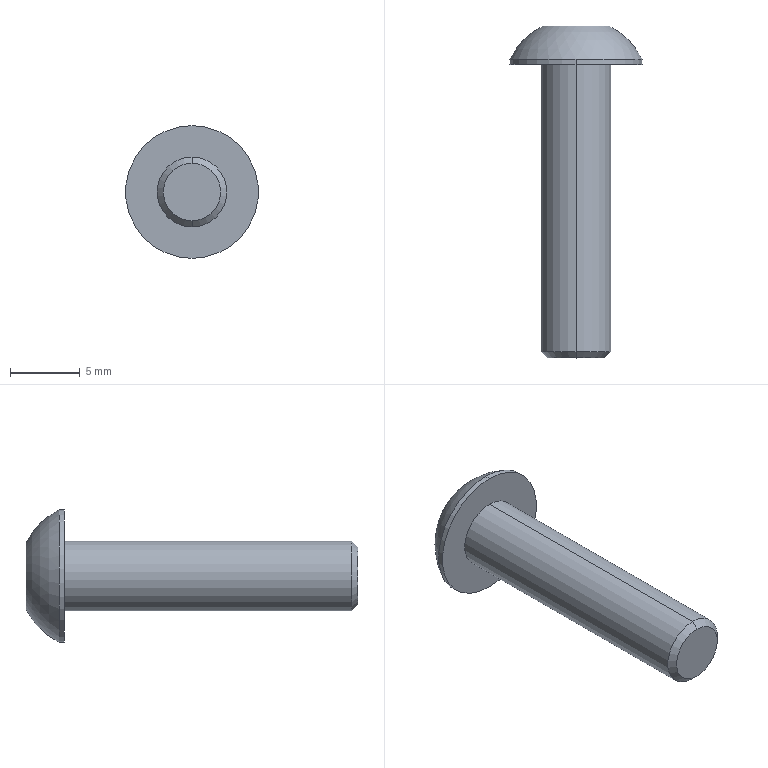Part | SolidWorks | features BaseBody 1 | 1 solid | 17 faces | box 9.5 x 23.75 x 9.5 mm | volume 537.038 mm3 | plane 10 | cylinder 4 | cone 2 | sphere 1 | commonest cylinder face diameters 5 x2 9.5 x2
STEP:
#1=CARTESIAN_POINT('',(0.,-21.,-2.055));
#2=VERTEX_POINT('',#1);
#3=CARTESIAN_POINT('',(0.,-21.,2.055));
#4=VERTEX_POINT('',#3);
#5=CARTESIAN_POINT('',(0.,-21.,0.));
#6=DIRECTION('',(0.,-1.,0.));
#7=DIRECTION('',(0.,0.,-1.));
#8=AXIS2_PLACEMENT_3D('',#5,#6,#7);
#9=CIRCLE('',#8,2.055);
#10=EDGE_CURVE('',#2,#4,#9,.T.);
#11=ORIENTED_EDGE('',*,*,#10,.F.);
#12=CARTESIAN_POINT('',(0.,-20.555,-2.5));
#13=VERTEX_POINT('',#12);
#14=CARTESIAN_POINT('',(0.,-21.,-2.055));
#15=DIRECTION('',(0.,0.7071,-0.7071));
#16=VECTOR('',#15,1000.);
#17=LINE('',#14,#16);
#18=EDGE_CURVE('',#2,#13,#17,.T.);
#19=ORIENTED_EDGE('',*,*,#18,.T.);
#20=CARTESIAN_POINT('',(0.,-20.555,2.5));
#21=VERTEX_POINT('',#20);
#22=CARTESIAN_POINT('',(0.,-20.555,0.));
#23=DIRECTION('',(0.,1.,0.));
#24=DIRECTION('',(0.,0.,-1.));
#25=AXIS2_PLACEMENT_3D('',#22,#23,#24);
#26=CIRCLE('',#25,2.5);
#27=EDGE_CURVE('',#21,#13,#26,.T.);
#28=ORIENTED_EDGE('',*,*,#27,.F.);
#29=CARTESIAN_POINT('',(0.,-21.,2.055));
#30=DIRECTION('',(0.,0.7071,0.7071));
#31=VECTOR('',#30,1000.);
#32=LINE('',#29,#31);
#33=EDGE_CURVE('',#4,#21,#32,.T.);
#34=ORIENTED_EDGE('',*,*,#33,.F.);
#35=EDGE_LOOP('',(#11,#19,#28,#34));
#36=FACE_OUTER_BOUND('',#35,.T.);
#37=CARTESIAN_POINT('',(0.,-21.,0.));
#38=DIRECTION('',(0.,1.,0.));
#39=DIRECTION('',(0.,0.,1.));
#40=AXIS2_PLACEMENT_3D('',#37,#38,#39);
#41=CONICAL_SURFACE('',#40,2.055,0.7854);
#42=ADVANCED_FACE('',(#36),#41,.T.);
#43=ORIENTED_EDGE('',*,*,#27,.T.);
#44=CARTESIAN_POINT('',(0.,0.,-2.5));
#45=VERTEX_POINT('',#44);
#46=CARTESIAN_POINT('',(0.,-21.,-2.5));
#47=DIRECTION('',(0.,1.,0.));
#48=VECTOR('',#47,1000.);
#49=LINE('',#46,#48);
#50=EDGE_CURVE('',#13,#45,#49,.T.);
#51=ORIENTED_EDGE('',*,*,#50,.T.);
#52=CARTESIAN_POINT('',(0.,0.,2.5));
#53=VERTEX_POINT('',#52);
#54=CARTESIAN_POINT('',(0.,0.,0.));
#55=DIRECTION('',(0.,-1.,0.));
#56=DIRECTION('',(0.,0.,1.));
#57=AXIS2_PLACEMENT_3D('',#54,#55,#56);
#58=CIRCLE('',#57,2.5);
#59=EDGE_CURVE('',#45,#53,#58,.T.);
#60=ORIENTED_EDGE('',*,*,#59,.T.);
#61=CARTESIAN_POINT('',(0.,-21.,2.5));
#62=DIRECTION('',(0.,1.,0.));
#63=VECTOR('',#62,1000.);
#64=LINE('',#61,#63);
#65=EDGE_CURVE('',#21,#53,#64,.T.);
#66=ORIENTED_EDGE('',*,*,#65,.F.);
#67=EDGE_LOOP('',(#43,#51,#60,#66));
#68=FACE_OUTER_BOUND('',#67,.T.);
#69=CARTESIAN_POINT('',(0.,-21.,0.));
#70=DIRECTION('',(0.,1.,0.));
#71=DIRECTION('',(0.,0.,1.));
#72=AXIS2_PLACEMENT_3D('',#69,#70,#71);
#73=CYLINDRICAL_SURFACE('',#72,2.5);
#74=ADVANCED_FACE('',(#68),#73,.T.);
#75=CARTESIAN_POINT('',(0.,0.38,-4.75));
#76=VERTEX_POINT('',#75);
#77=CARTESIAN_POINT('',(0.,0.38,4.75));
#78=VERTEX_POINT('',#77);
#79=CARTESIAN_POINT('',(0.,0.38,0.));
#80=DIRECTION('',(0.,-1.,0.));
#81=DIRECTION('',(0.,0.,-1.));
#82=AXIS2_PLACEMENT_3D('',#79,#80,#81);
#83=CIRCLE('',#82,4.75);
#84=EDGE_CURVE('',#76,#78,#83,.T.);
#85=ORIENTED_EDGE('',*,*,#84,.T.);
#86=CARTESIAN_POINT('',(0.,0.,4.75));
#87=VERTEX_POINT('',#86);
#88=CARTESIAN_POINT('',(0.,2.75,4.75));
#89=DIRECTION('',(0.,-1.,0.));
#90=VECTOR('',#89,1000.);
#91=LINE('',#88,#90);
#92=EDGE_CURVE('',#78,#87,#91,.T.);
#93=ORIENTED_EDGE('',*,*,#92,.T.);
#94=CARTESIAN_POINT('',(0.,0.,-4.75));
#95=VERTEX_POINT('',#94);
#96=CARTESIAN_POINT('',(0.,0.,0.));
#97=DIRECTION('',(0.,1.,0.));
#98=DIRECTION('',(0.,0.,1.));
#99=AXIS2_PLACEMENT_3D('',#96,#97,#98);
#100=CIRCLE('',#99,4.75);
#101=EDGE_CURVE('',#87,#95,#100,.T.);
#102=ORIENTED_EDGE('',*,*,#101,.T.);
#103=CARTESIAN_POINT('',(0.,2.75,-4.75));
#104=DIRECTION('',(0.,-1.,0.));
#105=VECTOR('',#104,1000.);
#106=LINE('',#103,#105);
#107=EDGE_CURVE('',#76,#95,#106,.T.);
#108=ORIENTED_EDGE('',*,*,#107,.F.);
#109=EDGE_LOOP('',(#85,#93,#102,#108));
#110=FACE_OUTER_BOUND('',#109,.T.);
#111=CARTESIAN_POINT('',(0.,2.75,0.));
#112=DIRECTION('',(0.,-1.,0.));
#113=DIRECTION('',(0.,0.,-1.));
#114=AXIS2_PLACEMENT_3D('',#111,#112,#113);
#115=CYLINDRICAL_SURFACE('',#114,4.75);
#116=ADVANCED_FACE('',(#110),#115,.T.);
#117=CARTESIAN_POINT('',(0.8862,2.75,1.535));
#118=VERTEX_POINT('',#117);
#119=CARTESIAN_POINT('',(1.772,2.75,0.));
#120=VERTEX_POINT('',#119);
#121=CARTESIAN_POINT('',(0.8862,2.75,1.535));
#122=DIRECTION('',(0.5,0.,-0.866));
#123=VECTOR('',#122,1000.);
#124=LINE('',#121,#123);
#125=EDGE_CURVE('',#118,#120,#124,.T.);
#126=ORIENTED_EDGE('',*,*,#125,.F.);
#127=CARTESIAN_POINT('',(-0.8862,2.75,1.535));
#128=VERTEX_POINT('',#127);
#129=CARTESIAN_POINT('',(-0.8862,2.75,1.535));
#130=DIRECTION('',(1.,0.,0.));
#131=VECTOR('',#130,1000.);
#132=LINE('',#129,#131);
#133=EDGE_CURVE('',#128,#118,#132,.T.);
#134=ORIENTED_EDGE('',*,*,#133,.F.);
#135=CARTESIAN_POINT('',(-1.772,2.75,0.));
#136=VERTEX_POINT('',#135);
#137=CARTESIAN_POINT('',(-1.772,2.75,0.));
#138=DIRECTION('',(0.5,0.,0.866));
#139=VECTOR('',#138,1000.);
#140=LINE('',#137,#139);
#141=EDGE_CURVE('',#136,#128,#140,.T.);
#142=ORIENTED_EDGE('',*,*,#141,.F.);
#143=CARTESIAN_POINT('',(-0.8862,2.75,-1.535));
#144=VERTEX_POINT('',#143);
#145=CARTESIAN_POINT('',(-0.8862,2.75,-1.535));
#146=DIRECTION('',(-0.5,0.,0.866));
#147=VECTOR('',#146,1000.);
#148=LINE('',#145,#147);
#149=EDGE_CURVE('',#144,#136,#148,.T.);
#150=ORIENTED_EDGE('',*,*,#149,.F.);
#151=CARTESIAN_POINT('',(0.8862,2.75,-1.535));
#152=VERTEX_POINT('',#151);
#153=CARTESIAN_POINT('',(0.8862,2.75,-1.535));
#154=DIRECTION('',(-1.,0.,0.));
#155=VECTOR('',#154,1000.);
#156=LINE('',#153,#155);
#157=EDGE_CURVE('',#152,#144,#156,.T.);
#158=ORIENTED_EDGE('',*,*,#157,.F.);
#159=CARTESIAN_POINT('',(1.772,2.75,0.));
#160=DIRECTION('',(-0.5,0.,-0.866));
#161=VECTOR('',#160,1000.);
#162=LINE('',#159,#161);
#163=EDGE_CURVE('',#120,#152,#162,.T.);
#164=ORIENTED_EDGE('',*,*,#163,.F.);
#165=EDGE_LOOP('',(#126,#134,#142,#150,#158,#164));
#166=FACE_BOUND('',#165,.T.);
#167=CARTESIAN_POINT('',(0.,2.75,-2.375));
#168=VERTEX_POINT('',#167);
#169=CARTESIAN_POINT('',(0.,2.75,2.375));
#170=VERTEX_POINT('',#169);
#171=CARTESIAN_POINT('',(0.,2.75,0.));
#172=DIRECTION('',(0.,-1.,0.));
#173=DIRECTION('',(0.,0.,-1.));
#174=AXIS2_PLACEMENT_3D('',#171,#172,#173);
#175=CIRCLE('',#174,2.375);
#176=EDGE_CURVE('',#168,#170,#175,.T.);
#177=ORIENTED_EDGE('',*,*,#176,.F.);
#178=CARTESIAN_POINT('',(0.,2.75,0.));
#179=DIRECTION('',(0.,-1.,0.));
#180=DIRECTION('',(0.,0.,-1.));
#181=AXIS2_PLACEMENT_3D('',#178,#179,#180);
#182=CIRCLE('',#181,2.375);
#183=EDGE_CURVE('',#170,#168,#182,.T.);
#184=ORIENTED_EDGE('',*,*,#183,.F.);
#185=EDGE_LOOP('',(#177,#184));
#186=FACE_OUTER_BOUND('',#185,.T.);
#187=CARTESIAN_POINT('',(0.,2.75,0.));
#188=DIRECTION('',(0.,1.,0.));
#189=DIRECTION('',(1.,0.,0.));
#190=AXIS2_PLACEMENT_3D('',#187,#188,#189);
#191=PLANE('',#190);
#192=ADVANCED_FACE('',(#166,#186),#191,.T.);
#193=ORIENTED_EDGE('',*,*,#125,.T.);
#194=CARTESIAN_POINT('',(1.772,1.19,0.));
#195=VERTEX_POINT('',#194);
#196=CARTESIAN_POINT('',(1.772,1.19,0.));
#197=DIRECTION('',(0.,1.,0.));
#198=VECTOR('',#197,1000.);
#199=LINE('',#196,#198);
#200=EDGE_CURVE('',#195,#120,#199,.T.);
#201=ORIENTED_EDGE('',*,*,#200,.F.);
#202=CARTESIAN_POINT('',(0.8862,1.19,1.535));
#203=VERTEX_POINT('',#202);
#204=CARTESIAN_POINT('',(0.8862,1.19,1.535));
#205=DIRECTION('',(0.5,0.,-0.866));
#206=VECTOR('',#205,1000.);
#207=LINE('',#204,#206);
#208=EDGE_CURVE('',#203,#195,#207,.T.);
#209=ORIENTED_EDGE('',*,*,#208,.F.);
#210=CARTESIAN_POINT('',(0.8862,1.19,1.535));
#211=DIRECTION('',(0.,1.,0.));
#212=VECTOR('',#211,1000.);
#213=LINE('',#210,#212);
#214=EDGE_CURVE('',#203,#118,#213,.T.);
#215=ORIENTED_EDGE('',*,*,#214,.T.);
#216=EDGE_LOOP('',(#193,#201,#209,#215));
#217=FACE_OUTER_BOUND('',#216,.T.);
#218=CARTESIAN_POINT('',(0.8862,1.19,1.535));
#219=DIRECTION('',(0.866,0.,0.5));
#220=DIRECTION('',(0.,-1.,0.));
#221=AXIS2_PLACEMENT_3D('',#218,#219,#220);
#222=PLANE('',#221);
#223=ADVANCED_FACE('',(#217),#222,.F.);
#224=ORIENTED_EDGE('',*,*,#133,.T.);
#225=ORIENTED_EDGE('',*,*,#214,.F.);
#226=CARTESIAN_POINT('',(-0.8862,1.19,1.535));
#227=VERTEX_POINT('',#226);
#228=CARTESIAN_POINT('',(-0.8862,1.19,1.535));
#229=DIRECTION('',(1.,0.,0.));
#230=VECTOR('',#229,1000.);
#231=LINE('',#228,#230);
#232=EDGE_CURVE('',#227,#203,#231,.T.);
#233=ORIENTED_EDGE('',*,*,#232,.F.);
#234=CARTESIAN_POINT('',(-0.8862,1.19,1.535));
#235=DIRECTION('',(0.,1.,0.));
#236=VECTOR('',#235,1000.);
#237=LINE('',#234,#236);
#238=EDGE_CURVE('',#227,#128,#237,.T.);
#239=ORIENTED_EDGE('',*,*,#238,.T.);
#240=EDGE_LOOP('',(#224,#225,#233,#239));
#241=FACE_OUTER_BOUND('',#240,.T.);
#242=CARTESIAN_POINT('',(-0.8862,1.19,1.535));
#243=DIRECTION('',(0.,0.,1.));
#244=DIRECTION('',(1.,0.,0.));
#245=AXIS2_PLACEMENT_3D('',#242,#243,#244);
#246=PLANE('',#245);
#247=ADVANCED_FACE('',(#241),#246,.F.);
#248=ORIENTED_EDGE('',*,*,#141,.T.);
#249=ORIENTED_EDGE('',*,*,#238,.F.);
#250=CARTESIAN_POINT('',(-1.772,1.19,0.));
#251=VERTEX_POINT('',#250);
#252=CARTESIAN_POINT('',(-1.772,1.19,0.));
#253=DIRECTION('',(0.5,0.,0.866));
#254=VECTOR('',#253,1000.);
#255=LINE('',#252,#254);
#256=EDGE_CURVE('',#251,#227,#255,.T.);
#257=ORIENTED_EDGE('',*,*,#256,.F.);
#258=CARTESIAN_POINT('',(-1.772,1.19,0.));
#259=DIRECTION('',(0.,1.,0.));
#260=VECTOR('',#259,1000.);
#261=LINE('',#258,#260);
#262=EDGE_CURVE('',#251,#136,#261,.T.);
#263=ORIENTED_EDGE('',*,*,#262,.T.);
#264=EDGE_LOOP('',(#248,#249,#257,#263));
#265=FACE_OUTER_BOUND('',#264,.T.);
#266=CARTESIAN_POINT('',(-1.772,1.19,0.));
#267=DIRECTION('',(-0.866,0.,0.5));
#268=DIRECTION('',(0.,1.,0.));
#269=AXIS2_PLACEMENT_3D('',#266,#267,#268);
#270=PLANE('',#269);
#271=ADVANCED_FACE('',(#265),#270,.F.);
#272=ORIENTED_EDGE('',*,*,#149,.T.);
#273=ORIENTED_EDGE('',*,*,#262,.F.);
#274=CARTESIAN_POINT('',(-0.8862,1.19,-1.535));
#275=VERTEX_POINT('',#274);
#276=CARTESIAN_POINT('',(-0.8862,1.19,-1.535));
#277=DIRECTION('',(-0.5,0.,0.866));
#278=VECTOR('',#277,1000.);
#279=LINE('',#276,#278);
#280=EDGE_CURVE('',#275,#251,#279,.T.);
#281=ORIENTED_EDGE('',*,*,#280,.F.);
#282=CARTESIAN_POINT('',(-0.8862,1.19,-1.535));
#283=DIRECTION('',(0.,1.,0.));
#284=VECTOR('',#283,1000.);
#285=LINE('',#282,#284);
#286=EDGE_CURVE('',#275,#144,#285,.T.);
#287=ORIENTED_EDGE('',*,*,#286,.T.);
#288=EDGE_LOOP('',(#272,#273,#281,#287));
#289=FACE_OUTER_BOUND('',#288,.T.);
#290=CARTESIAN_POINT('',(-0.8862,1.19,-1.535));
#291=DIRECTION('',(-0.866,0.,-0.5));
#292=DIRECTION('',(-0.5,0.,0.866));
#293=AXIS2_PLACEMENT_3D('',#290,#291,#292);
#294=PLANE('',#293);
#295=ADVANCED_FACE('',(#289),#294,.F.);
#296=ORIENTED_EDGE('',*,*,#157,.T.);
#297=ORIENTED_EDGE('',*,*,#286,.F.);
#298=CARTESIAN_POINT('',(0.8862,1.19,-1.535));
#299=VERTEX_POINT('',#298);
#300=CARTESIAN_POINT('',(0.8862,1.19,-1.535));
#301=DIRECTION('',(-1.,0.,0.));
#302=VECTOR('',#301,1000.);
#303=LINE('',#300,#302);
#304=EDGE_CURVE('',#299,#275,#303,.T.);
#305=ORIENTED_EDGE('',*,*,#304,.F.);
#306=CARTESIAN_POINT('',(0.8862,1.19,-1.535));
#307=DIRECTION('',(0.,1.,0.));
#308=VECTOR('',#307,1000.);
#309=LINE('',#306,#308);
#310=EDGE_CURVE('',#299,#152,#309,.T.);
#311=ORIENTED_EDGE('',*,*,#310,.T.);
#312=EDGE_LOOP('',(#296,#297,#305,#311));
#313=FACE_OUTER_BOUND('',#312,.T.);
#314=CARTESIAN_POINT('',(0.8862,1.19,-1.535));
#315=DIRECTION('',(0.,0.,-1.));
#316=DIRECTION('',(-1.,0.,0.));
#317=AXIS2_PLACEMENT_3D('',#314,#315,#316);
#318=PLANE('',#317);
#319=ADVANCED_FACE('',(#313),#318,.F.);
#320=ORIENTED_EDGE('',*,*,#163,.T.);
#321=ORIENTED_EDGE('',*,*,#310,.F.);
#322=CARTESIAN_POINT('',(1.772,1.19,0.));
#323=DIRECTION('',(-0.5,0.,-0.866));
#324=VECTOR('',#323,1000.);
#325=LINE('',#322,#324);
#326=EDGE_CURVE('',#195,#299,#325,.T.);
#327=ORIENTED_EDGE('',*,*,#326,.F.);
#328=ORIENTED_EDGE('',*,*,#200,.T.);
#329=EDGE_LOOP('',(#320,#321,#327,#328));
#330=FACE_OUTER_BOUND('',#329,.T.);
#331=CARTESIAN_POINT('',(1.772,1.19,0.));
#332=DIRECTION('',(0.866,0.,-0.5));
#333=DIRECTION('',(0.,-1.,0.));
#334=AXIS2_PLACEMENT_3D('',#331,#332,#333);
#335=PLANE('',#334);
#336=ADVANCED_FACE('',(#330),#335,.F.);
#337=ORIENTED_EDGE('',*,*,#208,.T.);
#338=ORIENTED_EDGE('',*,*,#326,.T.);
#339=ORIENTED_EDGE('',*,*,#304,.T.);
#340=ORIENTED_EDGE('',*,*,#280,.T.);
#341=ORIENTED_EDGE('',*,*,#256,.T.);
#342=ORIENTED_EDGE('',*,*,#232,.T.);
#343=EDGE_LOOP('',(#337,#338,#339,#340,#341,#342));
#344=FACE_OUTER_BOUND('',#343,.T.);
#345=CARTESIAN_POINT('',(0.,1.19,0.));
#346=DIRECTION('',(0.,1.,0.));
#347=DIRECTION('',(1.,0.,0.));
#348=AXIS2_PLACEMENT_3D('',#345,#346,#347);
#349=PLANE('',#348);
#350=ADVANCED_FACE('',(#344),#349,.T.);
#351=CARTESIAN_POINT('',(0.,-21.,0.));
#352=DIRECTION('',(0.,-1.,0.));
#353=DIRECTION('',(0.,0.,-1.));
#354=AXIS2_PLACEMENT_3D('',#351,#352,#353);
#355=CIRCLE('',#354,2.055);
#356=EDGE_CURVE('',#4,#2,#355,.T.);
#357=ORIENTED_EDGE('',*,*,#356,.T.);
#358=ORIENTED_EDGE('',*,*,#10,.T.);
#359=EDGE_LOOP('',(#357,#358));
#360=FACE_OUTER_BOUND('',#359,.T.);
#361=CARTESIAN_POINT('',(0.,-21.,0.));
#362=DIRECTION('',(0.,-1.,0.));
#363=DIRECTION('',(0.,0.,-1.));
#364=AXIS2_PLACEMENT_3D('',#361,#362,#363);
#365=PLANE('',#364);
#366=ADVANCED_FACE('',(#360),#365,.T.);
#367=CARTESIAN_POINT('',(0.,0.,0.));
#368=DIRECTION('',(0.,-1.,0.));
#369=DIRECTION('',(0.,0.,1.));
#370=AXIS2_PLACEMENT_3D('',#367,#368,#369);
#371=CIRCLE('',#370,2.5);
#372=EDGE_CURVE('',#53,#45,#371,.T.);
#373=ORIENTED_EDGE('',*,*,#372,.F.);
#374=ORIENTED_EDGE('',*,*,#59,.F.);
#375=EDGE_LOOP('',(#373,#374));
#376=FACE_BOUND('',#375,.T.);
#377=CARTESIAN_POINT('',(0.,0.,0.));
#378=DIRECTION('',(0.,1.,0.));
#379=DIRECTION('',(0.,0.,1.));
#380=AXIS2_PLACEMENT_3D('',#377,#378,#379);
#381=CIRCLE('',#380,4.75);
#382=EDGE_CURVE('',#95,#87,#381,.T.);
#383=ORIENTED_EDGE('',*,*,#382,.F.);
#384=ORIENTED_EDGE('',*,*,#101,.F.);
#385=EDGE_LOOP('',(#383,#384));
#386=FACE_OUTER_BOUND('',#385,.T.);
#387=CARTESIAN_POINT('',(0.,0.,0.));
#388=DIRECTION('',(0.,1.,0.));
#389=DIRECTION('',(1.,0.,0.));
#390=AXIS2_PLACEMENT_3D('',#387,#388,#389);
#391=PLANE('',#390);
#392=ADVANCED_FACE('',(#376,#386),#391,.F.);
#393=ORIENTED_EDGE('',*,*,#92,.F.);
#394=CARTESIAN_POINT('',(0.,0.38,0.));
#395=DIRECTION('',(0.,-1.,0.));
#396=DIRECTION('',(0.,0.,-1.));
#397=AXIS2_PLACEMENT_3D('',#394,#395,#396);
#398=CIRCLE('',#397,4.75);
#399=EDGE_CURVE('',#78,#76,#398,.T.);
#400=ORIENTED_EDGE('',*,*,#399,.T.);
#401=ORIENTED_EDGE('',*,*,#107,.T.);
#402=ORIENTED_EDGE('',*,*,#382,.T.);
#403=EDGE_LOOP('',(#393,#400,#401,#402));
#404=FACE_OUTER_BOUND('',#403,.T.);
#405=CARTESIAN_POINT('',(0.,2.75,0.));
#406=DIRECTION('',(0.,-1.,0.));
#407=DIRECTION('',(0.,0.,-1.));
#408=AXIS2_PLACEMENT_3D('',#405,#406,#407);
#409=CYLINDRICAL_SURFACE('',#408,4.75);
#410=ADVANCED_FACE('',(#404),#409,.T.);
#411=ORIENTED_EDGE('',*,*,#50,.F.);
#412=CARTESIAN_POINT('',(0.,-20.555,0.));
#413=DIRECTION('',(0.,1.,0.));
#414=DIRECTION('',(0.,0.,-1.));
#415=AXIS2_PLACEMENT_3D('',#412,#413,#414);
#416=CIRCLE('',#415,2.5);
#417=EDGE_CURVE('',#13,#21,#416,.T.);
#418=ORIENTED_EDGE('',*,*,#417,.T.);
#419=ORIENTED_EDGE('',*,*,#65,.T.);
#420=ORIENTED_EDGE('',*,*,#372,.T.);
#421=EDGE_LOOP('',(#411,#418,#419,#420));
#422=FACE_OUTER_BOUND('',#421,.T.);
#423=CARTESIAN_POINT('',(0.,-21.,0.));
#424=DIRECTION('',(0.,1.,0.));
#425=DIRECTION('',(0.,0.,1.));
#426=AXIS2_PLACEMENT_3D('',#423,#424,#425);
#427=CYLINDRICAL_SURFACE('',#426,2.5);
#428=ADVANCED_FACE('',(#422),#427,.T.);
#429=ORIENTED_EDGE('',*,*,#84,.F.);
#430=ORIENTED_EDGE('',*,*,#399,.F.);
#431=EDGE_LOOP('',(#429,#430));
#432=FACE_OUTER_BOUND('',#431,.T.);
#433=ORIENTED_EDGE('',*,*,#176,.T.);
#434=ORIENTED_EDGE('',*,*,#183,.T.);
#435=EDGE_LOOP('',(#433,#434));
#436=FACE_BOUND('',#435,.T.);
#437=CARTESIAN_POINT('',(0.,-2.005,0.));
#438=DIRECTION('',(0.,1.,0.));
#439=DIRECTION('',(1.,0.,0.));
#440=AXIS2_PLACEMENT_3D('',#437,#438,#439);
#441=SPHERICAL_SURFACE('',#440,5.315);
#442=ADVANCED_FACE('',(#432,#436),#441,.T.);
#443=ORIENTED_EDGE('',*,*,#18,.F.);
#444=ORIENTED_EDGE('',*,*,#356,.F.);
#445=ORIENTED_EDGE('',*,*,#33,.T.);
#446=ORIENTED_EDGE('',*,*,#417,.F.);
#447=EDGE_LOOP('',(#443,#444,#445,#446));
#448=FACE_OUTER_BOUND('',#447,.T.);
#449=CARTESIAN_POINT('',(0.,-21.,0.));
#450=DIRECTION('',(0.,1.,0.));
#451=DIRECTION('',(0.,0.,1.));
#452=AXIS2_PLACEMENT_3D('',#449,#450,#451);
#453=CONICAL_SURFACE('',#452,2.055,0.7854);
#454=ADVANCED_FACE('',(#448),#453,.T.);
#455=CLOSED_SHELL('',(#42,#74,#116,#192,#223,#247,#271,#295,#319,#336,#350,#366,#392,#410,#428,#442,#454));
#456=MANIFOLD_SOLID_BREP('',#455);
#457=CARTESIAN_POINT('',(0.,0.,0.));
#458=DIRECTION('',(0.,0.,1.));
#459=DIRECTION('',(1.,0.,0.));
#460=AXIS2_PLACEMENT_3D('',#457,#458,#459);
#461=(LENGTH_UNIT()NAMED_UNIT(*)SI_UNIT(.MILLI.,.METRE.));
#462=UNCERTAINTY_MEASURE_WITH_UNIT(LENGTH_MEASURE(0.00001),#461,'','');
#463=(NAMED_UNIT(*)PLANE_ANGLE_UNIT()SI_UNIT($,.RADIAN.));
#464=(NAMED_UNIT(*)SI_UNIT($,.STERADIAN.)SOLID_ANGLE_UNIT());
#465=(GEOMETRIC_REPRESENTATION_CONTEXT(3)GLOBAL_UNCERTAINTY_ASSIGNED_CONTEXT((#462))GLOBAL_UNIT_ASSIGNED_CONTEXT((#461,#463,#464))REPRESENTATION_CONTEXT('',''));
#466=ADVANCED_BREP_SHAPE_REPRESENTATION('',(#456,#460),#465);